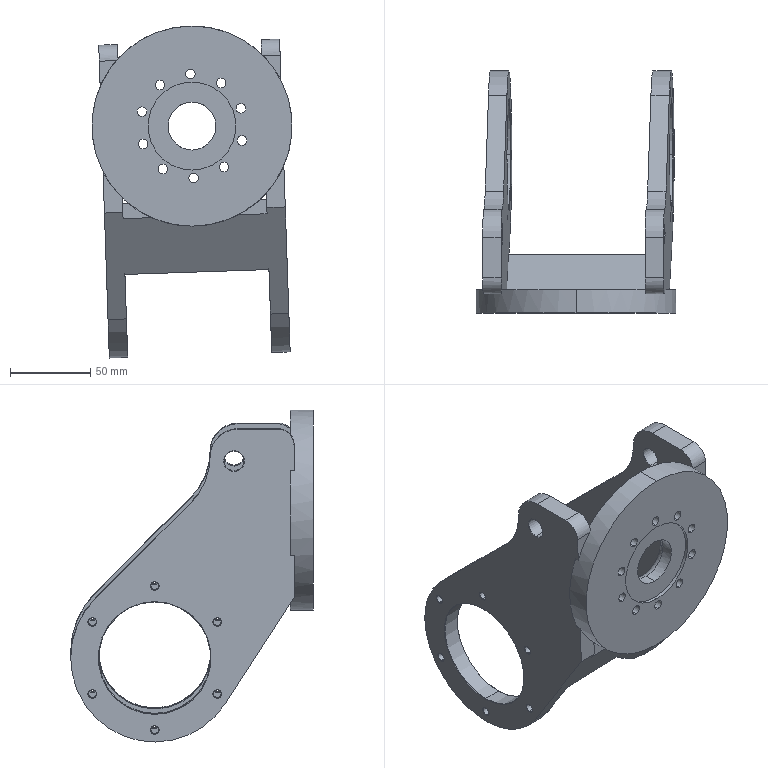Part | STEP file | 2026.6.15-Main Assembly图.sldasm-Part-86 | 1 solid | 156 faces | box 125 x 151.535 x 207.355 mm | volume 471937 mm3 | cylinder 67 | cone 62 | plane 25 | torus 2 | commonest cylinder face diameters 5 x24 6 x20 12.5 x4 70 x4 105 x3 20 x2